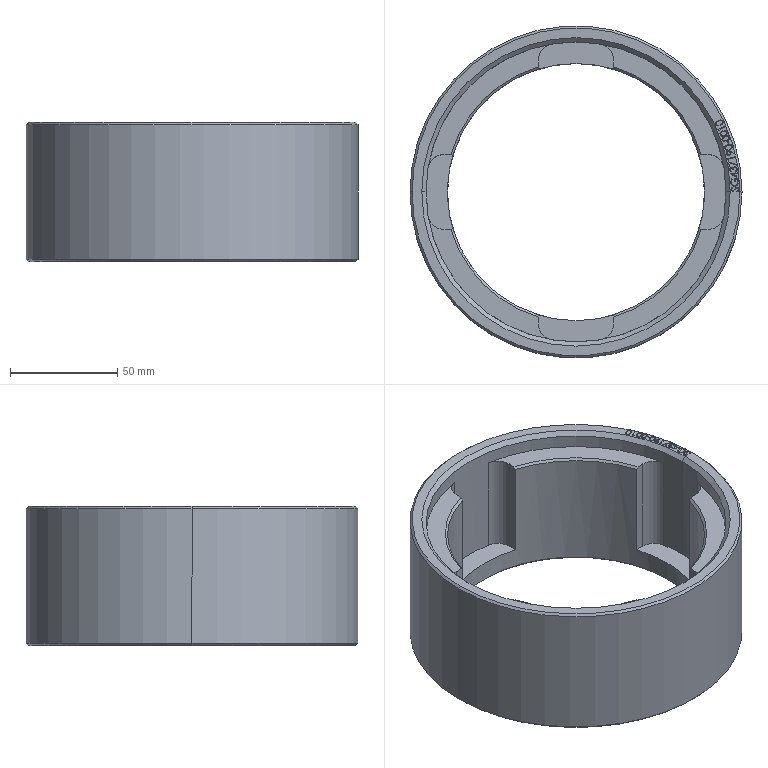Part | STEP file | Clearance measuring fixture seat-market | 1 solid | 205 faces | box 155 x 155 x 65 mm | volume 392527 mm3 | plane 88 | spline 83 | cylinder 22 | cone 12 | commonest cylinder face diameters 5 x8 15 x8 120 x2 140 x2 155 x2